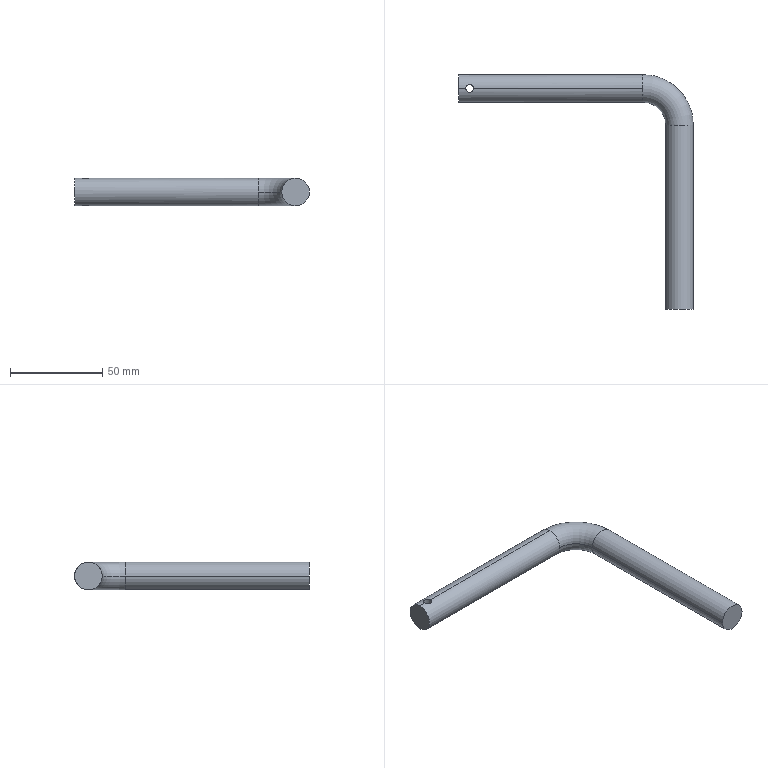Part | SolidWorks | features ICE 1, Sweep 1 | 1 solid | 10 faces | box 127.5 x 127.5 x 15 mm | volume 40689 mm3 | cylinder 6 | torus 2 | plane 2 | commonest cylinder face diameters 15 x4 4.2 x2
STEP:
#1=CARTESIAN_POINT('',(100.,7.5,0.));
#2=VERTEX_POINT('',#1);
#3=CARTESIAN_POINT('',(100.,0.,-7.5));
#4=VERTEX_POINT('',#3);
#5=CARTESIAN_POINT('',(100.,0.,0.));
#6=DIRECTION('',(-1.,0.,0.));
#7=DIRECTION('',(0.,-1.,0.));
#8=AXIS2_PLACEMENT_3D('',#5,#6,#7);
#9=CIRCLE('',#8,7.5);
#10=EDGE_CURVE('',#2,#4,#9,.T.);
#11=ORIENTED_EDGE('',*,*,#10,.F.);
#12=CARTESIAN_POINT('',(127.5,-20.,0.));
#13=VERTEX_POINT('',#12);
#14=CARTESIAN_POINT('',(100.,-20.,0.));
#15=DIRECTION('',(0.,0.,-1.));
#16=DIRECTION('',(-1.,0.,0.));
#17=AXIS2_PLACEMENT_3D('',#14,#15,#16);
#18=CIRCLE('',#17,27.5);
#19=EDGE_CURVE('',#2,#13,#18,.T.);
#20=ORIENTED_EDGE('',*,*,#19,.T.);
#21=CARTESIAN_POINT('',(112.5,-20.,0.));
#22=VERTEX_POINT('',#21);
#23=CARTESIAN_POINT('',(120.,-20.,0.));
#24=DIRECTION('',(0.,1.,0.));
#25=DIRECTION('',(-1.,0.,0.));
#26=AXIS2_PLACEMENT_3D('',#23,#24,#25);
#27=CIRCLE('',#26,7.5);
#28=EDGE_CURVE('',#13,#22,#27,.T.);
#29=ORIENTED_EDGE('',*,*,#28,.T.);
#30=CARTESIAN_POINT('',(100.,-7.5,0.));
#31=VERTEX_POINT('',#30);
#32=CARTESIAN_POINT('',(100.,-20.,0.));
#33=DIRECTION('',(0.,0.,-1.));
#34=DIRECTION('',(-1.,0.,0.));
#35=AXIS2_PLACEMENT_3D('',#32,#33,#34);
#36=CIRCLE('',#35,12.5);
#37=EDGE_CURVE('',#31,#22,#36,.T.);
#38=ORIENTED_EDGE('',*,*,#37,.F.);
#39=CARTESIAN_POINT('',(100.,0.,0.));
#40=DIRECTION('',(-1.,0.,0.));
#41=DIRECTION('',(0.,-1.,0.));
#42=AXIS2_PLACEMENT_3D('',#39,#40,#41);
#43=CIRCLE('',#42,7.5);
#44=EDGE_CURVE('',#4,#31,#43,.T.);
#45=ORIENTED_EDGE('',*,*,#44,.F.);
#46=EDGE_LOOP('',(#11,#20,#29,#38,#45));
#47=FACE_OUTER_BOUND('',#46,.T.);
#48=CARTESIAN_POINT('',(100.,-20.,0.));
#49=DIRECTION('',(0.,0.,-1.));
#50=DIRECTION('',(-1.,0.,0.));
#51=AXIS2_PLACEMENT_3D('',#48,#49,#50);
#52=TOROIDAL_SURFACE('',#51,20.,7.5);
#53=ADVANCED_FACE('',(#47),#52,.T.);
#54=CARTESIAN_POINT('',(3.9,0.,-7.5));
#55=VERTEX_POINT('',#54);
#56=CARTESIAN_POINT('',(8.1,0.,-7.5));
#57=VERTEX_POINT('',#56);
#58=CARTESIAN_POINT('',(3.9,0.,-7.5));
#59=CARTESIAN_POINT('',(3.9,-0.1395,-7.5));
#60=CARTESIAN_POINT('',(3.914,-0.2765,-7.496));
#61=CARTESIAN_POINT('',(3.968,-0.5459,-7.481));
#62=CARTESIAN_POINT('',(4.008,-0.6797,-7.47));
#63=CARTESIAN_POINT('',(4.114,-0.9337,-7.443));
#64=CARTESIAN_POINT('',(4.179,-1.054,-7.426));
#65=CARTESIAN_POINT('',(4.331,-1.282,-7.391));
#66=CARTESIAN_POINT('',(4.419,-1.389,-7.371));
#67=CARTESIAN_POINT('',(4.708,-1.678,-7.313));
#68=CARTESIAN_POINT('',(4.941,-1.834,-7.273));
#69=CARTESIAN_POINT('',(5.32,-1.992,-7.231));
#70=CARTESIAN_POINT('',(5.453,-2.032,-7.219));
#71=CARTESIAN_POINT('',(5.725,-2.086,-7.204));
#72=CARTESIAN_POINT('',(5.861,-2.1,-7.2));
#73=CARTESIAN_POINT('',(6.137,-2.1,-7.2));
#74=CARTESIAN_POINT('',(6.277,-2.086,-7.204));
#75=CARTESIAN_POINT('',(6.547,-2.032,-7.219));
#76=CARTESIAN_POINT('',(6.678,-1.992,-7.231));
#77=CARTESIAN_POINT('',(7.061,-1.833,-7.273));
#78=CARTESIAN_POINT('',(7.291,-1.679,-7.312));
#79=CARTESIAN_POINT('',(7.582,-1.387,-7.371));
#80=CARTESIAN_POINT('',(7.669,-1.282,-7.39));
#81=CARTESIAN_POINT('',(7.821,-1.055,-7.426));
#82=CARTESIAN_POINT('',(7.887,-0.9321,-7.443));
#83=CARTESIAN_POINT('',(7.992,-0.6788,-7.47));
#84=CARTESIAN_POINT('',(8.032,-0.5478,-7.481));
#85=CARTESIAN_POINT('',(8.086,-0.2769,-7.496));
#86=CARTESIAN_POINT('',(8.1,-0.1375,-7.5));
#87=CARTESIAN_POINT('',(8.1,0.,-7.5));
#88=B_SPLINE_CURVE_WITH_KNOTS('',3,(#58,#59,#60,#61,#62,#63,#64,#65,#66,#67,#68,#69,#70,#71,#72,#73,#74,#75,#76,#77,#78,#79,#80,#81,#82,#83,#84,#85,#86,#87),.UNSPECIFIED.,.F.,.F.,(4,2,2,2,2,2,2,2,2,2,2,2,2,2,4),(0.,0.0004124,0.0008248,0.001237,0.00165,0.002475,0.002887,0.003299,0.003712,0.004124,0.004949,0.005361,0.005774,0.006186,0.006599),.UNSPECIFIED.);
#89=EDGE_CURVE('',#55,#57,#88,.T.);
#90=ORIENTED_EDGE('',*,*,#89,.F.);
#91=CARTESIAN_POINT('',(3.9,0.,7.5));
#92=VERTEX_POINT('',#91);
#93=CARTESIAN_POINT('',(3.9,0.,-12.5));
#94=DIRECTION('',(0.,0.,1.));
#95=VECTOR('',#94,1000.);
#96=LINE('',#93,#95);
#97=EDGE_CURVE('',#55,#92,#96,.T.);
#98=ORIENTED_EDGE('',*,*,#97,.T.);
#99=CARTESIAN_POINT('',(8.1,0.,7.5));
#100=VERTEX_POINT('',#99);
#101=CARTESIAN_POINT('',(8.1,0.,7.5));
#102=CARTESIAN_POINT('',(8.1,-0.1395,7.5));
#103=CARTESIAN_POINT('',(8.086,-0.2765,7.496));
#104=CARTESIAN_POINT('',(8.032,-0.5459,7.481));
#105=CARTESIAN_POINT('',(7.992,-0.6797,7.47));
#106=CARTESIAN_POINT('',(7.886,-0.9337,7.443));
#107=CARTESIAN_POINT('',(7.821,-1.054,7.426));
#108=CARTESIAN_POINT('',(7.669,-1.282,7.391));
#109=CARTESIAN_POINT('',(7.581,-1.389,7.371));
#110=CARTESIAN_POINT('',(7.292,-1.678,7.313));
#111=CARTESIAN_POINT('',(7.059,-1.834,7.273));
#112=CARTESIAN_POINT('',(6.68,-1.992,7.231));
#113=CARTESIAN_POINT('',(6.547,-2.032,7.219));
#114=CARTESIAN_POINT('',(6.275,-2.086,7.204));
#115=CARTESIAN_POINT('',(6.139,-2.1,7.2));
#116=CARTESIAN_POINT('',(5.863,-2.1,7.2));
#117=CARTESIAN_POINT('',(5.723,-2.086,7.204));
#118=CARTESIAN_POINT('',(5.453,-2.032,7.219));
#119=CARTESIAN_POINT('',(5.322,-1.992,7.231));
#120=CARTESIAN_POINT('',(4.939,-1.833,7.273));
#121=CARTESIAN_POINT('',(4.709,-1.679,7.312));
#122=CARTESIAN_POINT('',(4.418,-1.387,7.371));
#123=CARTESIAN_POINT('',(4.331,-1.282,7.39));
#124=CARTESIAN_POINT('',(4.179,-1.055,7.426));
#125=CARTESIAN_POINT('',(4.113,-0.9321,7.443));
#126=CARTESIAN_POINT('',(4.008,-0.6788,7.47));
#127=CARTESIAN_POINT('',(3.968,-0.5478,7.481));
#128=CARTESIAN_POINT('',(3.914,-0.2769,7.496));
#129=CARTESIAN_POINT('',(3.9,-0.1375,7.5));
#130=CARTESIAN_POINT('',(3.9,0.,7.5));
#131=B_SPLINE_CURVE_WITH_KNOTS('',3,(#101,#102,#103,#104,#105,#106,#107,#108,#109,#110,#111,#112,#113,#114,#115,#116,#117,#118,#119,#120,#121,#122,#123,#124,#125,#126,#127,#128,#129,#130),.UNSPECIFIED.,.F.,.F.,(4,2,2,2,2,2,2,2,2,2,2,2,2,2,4),(0.,0.0004124,0.0008248,0.001237,0.00165,0.002475,0.002887,0.003299,0.003712,0.004124,0.004949,0.005361,0.005774,0.006186,0.006599),.UNSPECIFIED.);
#132=EDGE_CURVE('',#100,#92,#131,.T.);
#133=ORIENTED_EDGE('',*,*,#132,.F.);
#134=CARTESIAN_POINT('',(8.1,0.,-12.5));
#135=DIRECTION('',(0.,0.,1.));
#136=VECTOR('',#135,1000.);
#137=LINE('',#134,#136);
#138=EDGE_CURVE('',#57,#100,#137,.T.);
#139=ORIENTED_EDGE('',*,*,#138,.F.);
#140=EDGE_LOOP('',(#90,#98,#133,#139));
#141=FACE_OUTER_BOUND('',#140,.T.);
#142=CARTESIAN_POINT('',(6.,0.,-12.5));
#143=DIRECTION('',(0.,0.,1.));
#144=DIRECTION('',(1.,0.,0.));
#145=AXIS2_PLACEMENT_3D('',#142,#143,#144);
#146=CYLINDRICAL_SURFACE('',#145,2.1);
#147=ADVANCED_FACE('',(#141),#146,.F.);
#148=CARTESIAN_POINT('',(120.,-20.,0.));
#149=DIRECTION('',(0.,1.,0.));
#150=DIRECTION('',(-1.,0.,0.));
#151=AXIS2_PLACEMENT_3D('',#148,#149,#150);
#152=CIRCLE('',#151,7.5);
#153=EDGE_CURVE('',#22,#13,#152,.T.);
#154=ORIENTED_EDGE('',*,*,#153,.F.);
#155=CARTESIAN_POINT('',(112.5,-120.,0.));
#156=VERTEX_POINT('',#155);
#157=CARTESIAN_POINT('',(112.5,-20.,0.));
#158=DIRECTION('',(0.,-1.,0.));
#159=VECTOR('',#158,1000.);
#160=LINE('',#157,#159);
#161=EDGE_CURVE('',#22,#156,#160,.T.);
#162=ORIENTED_EDGE('',*,*,#161,.T.);
#163=CARTESIAN_POINT('',(127.5,-120.,0.));
#164=VERTEX_POINT('',#163);
#165=CARTESIAN_POINT('',(120.,-120.,0.));
#166=DIRECTION('',(0.,1.,0.));
#167=DIRECTION('',(-1.,0.,0.));
#168=AXIS2_PLACEMENT_3D('',#165,#166,#167);
#169=CIRCLE('',#168,7.5);
#170=EDGE_CURVE('',#156,#164,#169,.T.);
#171=ORIENTED_EDGE('',*,*,#170,.T.);
#172=CARTESIAN_POINT('',(127.5,-20.,0.));
#173=DIRECTION('',(0.,-1.,0.));
#174=VECTOR('',#173,1000.);
#175=LINE('',#172,#174);
#176=EDGE_CURVE('',#13,#164,#175,.T.);
#177=ORIENTED_EDGE('',*,*,#176,.F.);
#178=EDGE_LOOP('',(#154,#162,#171,#177));
#179=FACE_OUTER_BOUND('',#178,.T.);
#180=CARTESIAN_POINT('',(120.,-20.,0.));
#181=DIRECTION('',(0.,-1.,0.));
#182=DIRECTION('',(1.,0.,0.));
#183=AXIS2_PLACEMENT_3D('',#180,#181,#182);
#184=CYLINDRICAL_SURFACE('',#183,7.5);
#185=ADVANCED_FACE('',(#179),#184,.T.);
#186=CARTESIAN_POINT('',(0.,0.,7.5));
#187=VERTEX_POINT('',#186);
#188=CARTESIAN_POINT('',(0.,0.,-7.5));
#189=VERTEX_POINT('',#188);
#190=CARTESIAN_POINT('',(0.,0.,0.));
#191=DIRECTION('',(-1.,0.,0.));
#192=DIRECTION('',(0.,-1.,0.));
#193=AXIS2_PLACEMENT_3D('',#190,#191,#192);
#194=CIRCLE('',#193,7.5);
#195=EDGE_CURVE('',#187,#189,#194,.T.);
#196=ORIENTED_EDGE('',*,*,#195,.F.);
#197=CARTESIAN_POINT('',(0.,0.,7.5));
#198=DIRECTION('',(1.,0.,0.));
#199=VECTOR('',#198,1000.);
#200=LINE('',#197,#199);
#201=EDGE_CURVE('',#187,#92,#200,.T.);
#202=ORIENTED_EDGE('',*,*,#201,.T.);
#203=CARTESIAN_POINT('',(3.9,0.,7.5));
#204=CARTESIAN_POINT('',(3.9,0.2749,7.5));
#205=CARTESIAN_POINT('',(3.956,0.5525,7.484));
#206=CARTESIAN_POINT('',(4.113,0.9321,7.443));
#207=CARTESIAN_POINT('',(4.179,1.055,7.426));
#208=CARTESIAN_POINT('',(4.331,1.282,7.39));
#209=CARTESIAN_POINT('',(4.418,1.388,7.371));
#210=CARTESIAN_POINT('',(4.612,1.581,7.332));
#211=CARTESIAN_POINT('',(4.719,1.669,7.312));
#212=CARTESIAN_POINT('',(4.945,1.821,7.276));
#213=CARTESIAN_POINT('',(5.066,1.886,7.259));
#214=CARTESIAN_POINT('',(5.321,1.992,7.231));
#215=CARTESIAN_POINT('',(5.453,2.032,7.219));
#216=CARTESIAN_POINT('',(5.722,2.086,7.204));
#217=CARTESIAN_POINT('',(5.861,2.1,7.2));
#218=CARTESIAN_POINT('',(6.138,2.1,7.2));
#219=CARTESIAN_POINT('',(6.275,2.086,7.204));
#220=CARTESIAN_POINT('',(6.545,2.033,7.219));
#221=CARTESIAN_POINT('',(6.679,1.992,7.231));
#222=CARTESIAN_POINT('',(7.059,1.834,7.273));
#223=CARTESIAN_POINT('',(7.292,1.678,7.312));
#224=CARTESIAN_POINT('',(7.581,1.389,7.371));
#225=CARTESIAN_POINT('',(7.669,1.283,7.39));
#226=CARTESIAN_POINT('',(7.821,1.054,7.426));
#227=CARTESIAN_POINT('',(7.886,0.9341,7.443));
#228=CARTESIAN_POINT('',(7.991,0.6811,7.47));
#229=CARTESIAN_POINT('',(8.032,0.5471,7.481));
#230=CARTESIAN_POINT('',(8.086,0.2768,7.496));
#231=CARTESIAN_POINT('',(8.1,0.1395,7.5));
#232=CARTESIAN_POINT('',(8.1,0.,7.5));
#233=B_SPLINE_CURVE_WITH_KNOTS('',3,(#203,#204,#205,#206,#207,#208,#209,#210,#211,#212,#213,#214,#215,#216,#217,#218,#219,#220,#221,#222,#223,#224,#225,#226,#227,#228,#229,#230,#231,#232),.UNSPECIFIED.,.F.,.F.,(4,2,2,2,2,2,2,2,2,2,2,2,2,2,4),(0.006599,0.007423,0.007836,0.008248,0.00866,0.009073,0.009485,0.009897,0.01031,0.01072,0.01155,0.01196,0.01237,0.01278,0.0132),.UNSPECIFIED.);
#234=EDGE_CURVE('',#92,#100,#233,.T.);
#235=ORIENTED_EDGE('',*,*,#234,.T.);
#236=CARTESIAN_POINT('',(100.,0.,7.5));
#237=VERTEX_POINT('',#236);
#238=CARTESIAN_POINT('',(0.,0.,7.5));
#239=DIRECTION('',(1.,0.,0.));
#240=VECTOR('',#239,1000.);
#241=LINE('',#238,#240);
#242=EDGE_CURVE('',#100,#237,#241,.T.);
#243=ORIENTED_EDGE('',*,*,#242,.T.);
#244=CARTESIAN_POINT('',(100.,0.,0.));
#245=DIRECTION('',(-1.,0.,0.));
#246=DIRECTION('',(0.,-1.,0.));
#247=AXIS2_PLACEMENT_3D('',#244,#245,#246);
#248=CIRCLE('',#247,7.5);
#249=EDGE_CURVE('',#237,#2,#248,.T.);
#250=ORIENTED_EDGE('',*,*,#249,.T.);
#251=ORIENTED_EDGE('',*,*,#10,.T.);
#252=CARTESIAN_POINT('',(0.,0.,-7.5));
#253=DIRECTION('',(1.,0.,0.));
#254=VECTOR('',#253,1000.);
#255=LINE('',#252,#254);
#256=EDGE_CURVE('',#57,#4,#255,.T.);
#257=ORIENTED_EDGE('',*,*,#256,.F.);
#258=CARTESIAN_POINT('',(8.1,0.,-7.5));
#259=CARTESIAN_POINT('',(8.1,0.2749,-7.5));
#260=CARTESIAN_POINT('',(8.044,0.5525,-7.484));
#261=CARTESIAN_POINT('',(7.887,0.9321,-7.443));
#262=CARTESIAN_POINT('',(7.821,1.055,-7.426));
#263=CARTESIAN_POINT('',(7.669,1.282,-7.39));
#264=CARTESIAN_POINT('',(7.582,1.388,-7.371));
#265=CARTESIAN_POINT('',(7.388,1.581,-7.332));
#266=CARTESIAN_POINT('',(7.281,1.669,-7.312));
#267=CARTESIAN_POINT('',(7.055,1.821,-7.276));
#268=CARTESIAN_POINT('',(6.934,1.886,-7.259));
#269=CARTESIAN_POINT('',(6.679,1.992,-7.231));
#270=CARTESIAN_POINT('',(6.547,2.032,-7.219));
#271=CARTESIAN_POINT('',(6.278,2.086,-7.204));
#272=CARTESIAN_POINT('',(6.139,2.1,-7.2));
#273=CARTESIAN_POINT('',(5.862,2.1,-7.2));
#274=CARTESIAN_POINT('',(5.725,2.086,-7.204));
#275=CARTESIAN_POINT('',(5.455,2.033,-7.219));
#276=CARTESIAN_POINT('',(5.321,1.992,-7.231));
#277=CARTESIAN_POINT('',(4.941,1.834,-7.273));
#278=CARTESIAN_POINT('',(4.708,1.678,-7.312));
#279=CARTESIAN_POINT('',(4.419,1.389,-7.371));
#280=CARTESIAN_POINT('',(4.331,1.283,-7.39));
#281=CARTESIAN_POINT('',(4.179,1.054,-7.426));
#282=CARTESIAN_POINT('',(4.114,0.9341,-7.443));
#283=CARTESIAN_POINT('',(4.009,0.6811,-7.47));
#284=CARTESIAN_POINT('',(3.968,0.5471,-7.481));
#285=CARTESIAN_POINT('',(3.914,0.2768,-7.496));
#286=CARTESIAN_POINT('',(3.9,0.1395,-7.5));
#287=CARTESIAN_POINT('',(3.9,0.,-7.5));
#288=B_SPLINE_CURVE_WITH_KNOTS('',3,(#258,#259,#260,#261,#262,#263,#264,#265,#266,#267,#268,#269,#270,#271,#272,#273,#274,#275,#276,#277,#278,#279,#280,#281,#282,#283,#284,#285,#286,#287),.UNSPECIFIED.,.F.,.F.,(4,2,2,2,2,2,2,2,2,2,2,2,2,2,4),(0.006599,0.007423,0.007836,0.008248,0.00866,0.009073,0.009485,0.009897,0.01031,0.01072,0.01155,0.01196,0.01237,0.01278,0.0132),.UNSPECIFIED.);
#289=EDGE_CURVE('',#57,#55,#288,.T.);
#290=ORIENTED_EDGE('',*,*,#289,.T.);
#291=CARTESIAN_POINT('',(0.,0.,-7.5));
#292=DIRECTION('',(1.,0.,0.));
#293=VECTOR('',#292,1000.);
#294=LINE('',#291,#293);
#295=EDGE_CURVE('',#189,#55,#294,.T.);
#296=ORIENTED_EDGE('',*,*,#295,.F.);
#297=EDGE_LOOP('',(#196,#202,#235,#243,#250,#251,#257,#290,#296));
#298=FACE_OUTER_BOUND('',#297,.T.);
#299=CARTESIAN_POINT('',(0.,0.,0.));
#300=DIRECTION('',(1.,0.,0.));
#301=DIRECTION('',(0.,0.,-1.));
#302=AXIS2_PLACEMENT_3D('',#299,#300,#301);
#303=CYLINDRICAL_SURFACE('',#302,7.5);
#304=ADVANCED_FACE('',(#298),#303,.T.);
#305=ORIENTED_EDGE('',*,*,#161,.F.);
#306=ORIENTED_EDGE('',*,*,#28,.F.);
#307=ORIENTED_EDGE('',*,*,#176,.T.);
#308=CARTESIAN_POINT('',(120.,-120.,0.));
#309=DIRECTION('',(0.,1.,0.));
#310=DIRECTION('',(-1.,0.,0.));
#311=AXIS2_PLACEMENT_3D('',#308,#309,#310);
#312=CIRCLE('',#311,7.5);
#313=EDGE_CURVE('',#164,#156,#312,.T.);
#314=ORIENTED_EDGE('',*,*,#313,.T.);
#315=EDGE_LOOP('',(#305,#306,#307,#314));
#316=FACE_OUTER_BOUND('',#315,.T.);
#317=CARTESIAN_POINT('',(120.,-20.,0.));
#318=DIRECTION('',(0.,-1.,0.));
#319=DIRECTION('',(1.,0.,0.));
#320=AXIS2_PLACEMENT_3D('',#317,#318,#319);
#321=CYLINDRICAL_SURFACE('',#320,7.5);
#322=ADVANCED_FACE('',(#316),#321,.T.);
#323=ORIENTED_EDGE('',*,*,#19,.F.);
#324=ORIENTED_EDGE('',*,*,#249,.F.);
#325=CARTESIAN_POINT('',(100.,0.,0.));
#326=DIRECTION('',(-1.,0.,0.));
#327=DIRECTION('',(0.,-1.,0.));
#328=AXIS2_PLACEMENT_3D('',#325,#326,#327);
#329=CIRCLE('',#328,7.5);
#330=EDGE_CURVE('',#31,#237,#329,.T.);
#331=ORIENTED_EDGE('',*,*,#330,.F.);
#332=ORIENTED_EDGE('',*,*,#37,.T.);
#333=ORIENTED_EDGE('',*,*,#153,.T.);
#334=EDGE_LOOP('',(#323,#324,#331,#332,#333));
#335=FACE_OUTER_BOUND('',#334,.T.);
#336=CARTESIAN_POINT('',(100.,-20.,0.));
#337=DIRECTION('',(0.,0.,-1.));
#338=DIRECTION('',(-1.,0.,0.));
#339=AXIS2_PLACEMENT_3D('',#336,#337,#338);
#340=TOROIDAL_SURFACE('',#339,20.,7.5);
#341=ADVANCED_FACE('',(#335),#340,.T.);
#342=ORIENTED_EDGE('',*,*,#201,.F.);
#343=CARTESIAN_POINT('',(0.,0.,0.));
#344=DIRECTION('',(-1.,0.,0.));
#345=DIRECTION('',(0.,-1.,0.));
#346=AXIS2_PLACEMENT_3D('',#343,#344,#345);
#347=CIRCLE('',#346,7.5);
#348=EDGE_CURVE('',#189,#187,#347,.T.);
#349=ORIENTED_EDGE('',*,*,#348,.F.);
#350=ORIENTED_EDGE('',*,*,#295,.T.);
#351=ORIENTED_EDGE('',*,*,#89,.T.);
#352=ORIENTED_EDGE('',*,*,#256,.T.);
#353=ORIENTED_EDGE('',*,*,#44,.T.);
#354=ORIENTED_EDGE('',*,*,#330,.T.);
#355=ORIENTED_EDGE('',*,*,#242,.F.);
#356=ORIENTED_EDGE('',*,*,#132,.T.);
#357=EDGE_LOOP('',(#342,#349,#350,#351,#352,#353,#354,#355,#356));
#358=FACE_OUTER_BOUND('',#357,.T.);
#359=CARTESIAN_POINT('',(0.,0.,0.));
#360=DIRECTION('',(1.,0.,0.));
#361=DIRECTION('',(0.,0.,-1.));
#362=AXIS2_PLACEMENT_3D('',#359,#360,#361);
#363=CYLINDRICAL_SURFACE('',#362,7.5);
#364=ADVANCED_FACE('',(#358),#363,.T.);
#365=ORIENTED_EDGE('',*,*,#313,.F.);
#366=ORIENTED_EDGE('',*,*,#170,.F.);
#367=EDGE_LOOP('',(#365,#366));
#368=FACE_OUTER_BOUND('',#367,.T.);
#369=CARTESIAN_POINT('',(120.,-120.,0.));
#370=DIRECTION('',(0.,1.,0.));
#371=DIRECTION('',(-1.,0.,0.));
#372=AXIS2_PLACEMENT_3D('',#369,#370,#371);
#373=PLANE('',#372);
#374=ADVANCED_FACE('',(#368),#373,.F.);
#375=ORIENTED_EDGE('',*,*,#348,.T.);
#376=ORIENTED_EDGE('',*,*,#195,.T.);
#377=EDGE_LOOP('',(#375,#376));
#378=FACE_OUTER_BOUND('',#377,.T.);
#379=CARTESIAN_POINT('',(0.,0.,0.));
#380=DIRECTION('',(-1.,0.,0.));
#381=DIRECTION('',(0.,-1.,0.));
#382=AXIS2_PLACEMENT_3D('',#379,#380,#381);
#383=PLANE('',#382);
#384=ADVANCED_FACE('',(#378),#383,.T.);
#385=ORIENTED_EDGE('',*,*,#97,.F.);
#386=ORIENTED_EDGE('',*,*,#289,.F.);
#387=ORIENTED_EDGE('',*,*,#138,.T.);
#388=ORIENTED_EDGE('',*,*,#234,.F.);
#389=EDGE_LOOP('',(#385,#386,#387,#388));
#390=FACE_OUTER_BOUND('',#389,.T.);
#391=CARTESIAN_POINT('',(6.,0.,-12.5));
#392=DIRECTION('',(0.,0.,1.));
#393=DIRECTION('',(1.,0.,0.));
#394=AXIS2_PLACEMENT_3D('',#391,#392,#393);
#395=CYLINDRICAL_SURFACE('',#394,2.1);
#396=ADVANCED_FACE('',(#390),#395,.F.);
#397=CLOSED_SHELL('',(#53,#147,#185,#304,#322,#341,#364,#374,#384,#396));
#398=MANIFOLD_SOLID_BREP('',#397);
#399=CARTESIAN_POINT('',(0.,0.,0.));
#400=DIRECTION('',(0.,0.,1.));
#401=DIRECTION('',(1.,0.,0.));
#402=AXIS2_PLACEMENT_3D('',#399,#400,#401);
#403=(LENGTH_UNIT()NAMED_UNIT(*)SI_UNIT(.MILLI.,.METRE.));
#404=UNCERTAINTY_MEASURE_WITH_UNIT(LENGTH_MEASURE(0.00001),#403,'','');
#405=(NAMED_UNIT(*)PLANE_ANGLE_UNIT()SI_UNIT($,.RADIAN.));
#406=(NAMED_UNIT(*)SI_UNIT($,.STERADIAN.)SOLID_ANGLE_UNIT());
#407=(GEOMETRIC_REPRESENTATION_CONTEXT(3)GLOBAL_UNCERTAINTY_ASSIGNED_CONTEXT((#404))GLOBAL_UNIT_ASSIGNED_CONTEXT((#403,#405,#406))REPRESENTATION_CONTEXT('',''));
#408=ADVANCED_BREP_SHAPE_REPRESENTATION('',(#398,#402),#407);